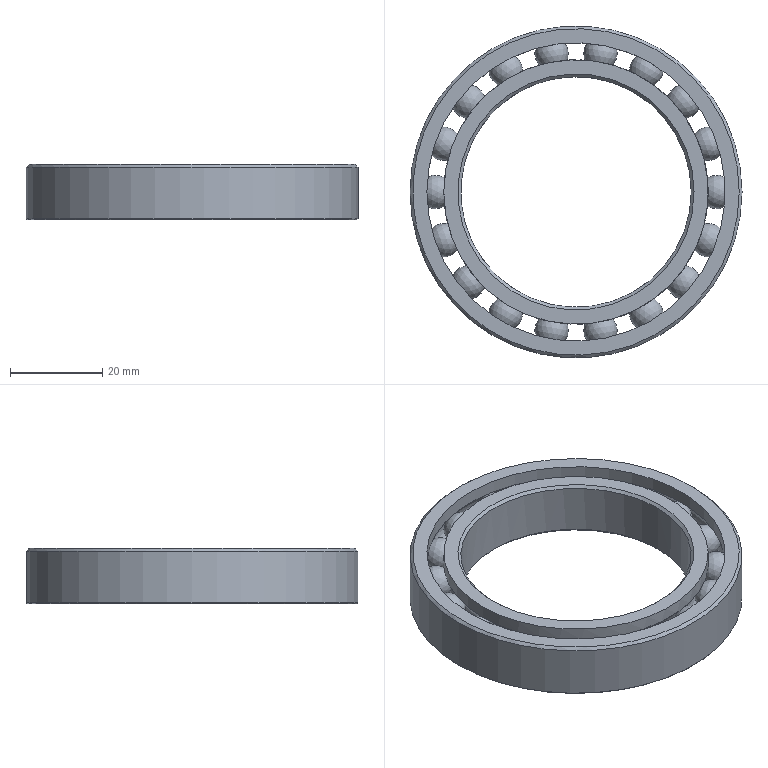Part | NX | 20 solids | 34 faces | box 72 x 72 x 12 mm | volume 17105 mm3 | sphere 18 | cylinder 5 | cone 5 | plane 4 | torus 2 | commonest cylinder face diameters 57.334 x2 50 x1 64.666 x1 72 x1
STEP:
#1=CARTESIAN_POINT('',(-5.296,-30.037,2.334));
#2=VERTEX_POINT('',#1);
#3=VERTEX_LOOP('',#2);
#4=FACE_BOUND('',#3,.T.);
#5=CARTESIAN_POINT('',(-5.296,-30.037,6.));
#6=DIRECTION('',(-0.1736,-0.9848,0.));
#7=DIRECTION('',(0.,0.,-1.));
#8=AXIS2_PLACEMENT_3D('',#5,#6,#7);
#9=SPHERICAL_SURFACE('',#8,3.666);
#10=ADVANCED_FACE('',(#4),#9,.T.);
#11=CLOSED_SHELL('',(#10));
#12=MANIFOLD_SOLID_BREP('',#11);
#13=CARTESIAN_POINT('',(5.296,30.037,2.334));
#14=VERTEX_POINT('',#13);
#15=VERTEX_LOOP('',#14);
#16=FACE_BOUND('',#15,.T.);
#17=CARTESIAN_POINT('',(5.296,30.037,6.));
#18=DIRECTION('',(0.1736,0.9848,0.));
#19=DIRECTION('',(0.,0.,-1.));
#20=AXIS2_PLACEMENT_3D('',#17,#18,#19);
#21=SPHERICAL_SURFACE('',#20,3.666);
#22=ADVANCED_FACE('',(#16),#21,.T.);
#23=CLOSED_SHELL('',(#22));
#24=MANIFOLD_SOLID_BREP('',#23);
#25=CARTESIAN_POINT('',(-23.364,19.605,2.334));
#26=VERTEX_POINT('',#25);
#27=VERTEX_LOOP('',#26);
#28=FACE_BOUND('',#27,.T.);
#29=CARTESIAN_POINT('',(-23.364,19.605,6.));
#30=DIRECTION('',(-0.766,0.6428,0.));
#31=DIRECTION('',(0.,0.,-1.));
#32=AXIS2_PLACEMENT_3D('',#29,#30,#31);
#33=SPHERICAL_SURFACE('',#32,3.666);
#34=ADVANCED_FACE('',(#28),#33,.T.);
#35=CLOSED_SHELL('',(#34));
#36=MANIFOLD_SOLID_BREP('',#35);
#37=CARTESIAN_POINT('',(28.661,10.432,2.334));
#38=VERTEX_POINT('',#37);
#39=VERTEX_LOOP('',#38);
#40=FACE_BOUND('',#39,.T.);
#41=CARTESIAN_POINT('',(28.661,10.432,6.));
#42=DIRECTION('',(0.9397,0.342,0.));
#43=DIRECTION('',(0.,0.,-1.));
#44=AXIS2_PLACEMENT_3D('',#41,#42,#43);
#45=SPHERICAL_SURFACE('',#44,3.666);
#46=ADVANCED_FACE('',(#40),#45,.T.);
#47=CLOSED_SHELL('',(#46));
#48=MANIFOLD_SOLID_BREP('',#47);
#49=CARTESIAN_POINT('',(-28.661,10.432,2.334));
#50=VERTEX_POINT('',#49);
#51=VERTEX_LOOP('',#50);
#52=FACE_BOUND('',#51,.T.);
#53=CARTESIAN_POINT('',(-28.661,10.432,6.));
#54=DIRECTION('',(-0.9397,0.342,0.));
#55=DIRECTION('',(0.,0.,-1.));
#56=AXIS2_PLACEMENT_3D('',#53,#54,#55);
#57=SPHERICAL_SURFACE('',#56,3.666);
#58=ADVANCED_FACE('',(#52),#57,.T.);
#59=CLOSED_SHELL('',(#58));
#60=MANIFOLD_SOLID_BREP('',#59);
#61=CARTESIAN_POINT('',(-23.364,-19.605,2.334));
#62=VERTEX_POINT('',#61);
#63=VERTEX_LOOP('',#62);
#64=FACE_BOUND('',#63,.T.);
#65=CARTESIAN_POINT('',(-23.364,-19.605,6.));
#66=DIRECTION('',(-0.766,-0.6428,0.));
#67=DIRECTION('',(0.,0.,-1.));
#68=AXIS2_PLACEMENT_3D('',#65,#66,#67);
#69=SPHERICAL_SURFACE('',#68,3.666);
#70=ADVANCED_FACE('',(#64),#69,.T.);
#71=CLOSED_SHELL('',(#70));
#72=MANIFOLD_SOLID_BREP('',#71);
#73=CARTESIAN_POINT('',(23.364,-19.605,2.334));
#74=VERTEX_POINT('',#73);
#75=VERTEX_LOOP('',#74);
#76=FACE_BOUND('',#75,.T.);
#77=CARTESIAN_POINT('',(23.364,-19.605,6.));
#78=DIRECTION('',(0.766,-0.6428,0.));
#79=DIRECTION('',(0.,0.,-1.));
#80=AXIS2_PLACEMENT_3D('',#77,#78,#79);
#81=SPHERICAL_SURFACE('',#80,3.666);
#82=ADVANCED_FACE('',(#76),#81,.T.);
#83=CLOSED_SHELL('',(#82));
#84=MANIFOLD_SOLID_BREP('',#83);
#85=CARTESIAN_POINT('',(15.25,-26.414,2.334));
#86=VERTEX_POINT('',#85);
#87=VERTEX_LOOP('',#86);
#88=FACE_BOUND('',#87,.T.);
#89=CARTESIAN_POINT('',(15.25,-26.414,6.));
#90=DIRECTION('',(0.5,-0.866,0.));
#91=DIRECTION('',(0.,0.,-1.));
#92=AXIS2_PLACEMENT_3D('',#89,#90,#91);
#93=SPHERICAL_SURFACE('',#92,3.666);
#94=ADVANCED_FACE('',(#88),#93,.T.);
#95=CLOSED_SHELL('',(#94));
#96=MANIFOLD_SOLID_BREP('',#95);
#97=CARTESIAN_POINT('',(-28.661,-10.432,2.334));
#98=VERTEX_POINT('',#97);
#99=VERTEX_LOOP('',#98);
#100=FACE_BOUND('',#99,.T.);
#101=CARTESIAN_POINT('',(-28.661,-10.432,6.));
#102=DIRECTION('',(-0.9397,-0.342,0.));
#103=DIRECTION('',(0.,0.,-1.));
#104=AXIS2_PLACEMENT_3D('',#101,#102,#103);
#105=SPHERICAL_SURFACE('',#104,3.666);
#106=ADVANCED_FACE('',(#100),#105,.T.);
#107=CLOSED_SHELL('',(#106));
#108=MANIFOLD_SOLID_BREP('',#107);
#109=CARTESIAN_POINT('',(-5.296,30.037,2.334));
#110=VERTEX_POINT('',#109);
#111=VERTEX_LOOP('',#110);
#112=FACE_BOUND('',#111,.T.);
#113=CARTESIAN_POINT('',(-5.296,30.037,6.));
#114=DIRECTION('',(-0.1736,0.9848,0.));
#115=DIRECTION('',(0.,0.,-1.));
#116=AXIS2_PLACEMENT_3D('',#113,#114,#115);
#117=SPHERICAL_SURFACE('',#116,3.666);
#118=ADVANCED_FACE('',(#112),#117,.T.);
#119=CLOSED_SHELL('',(#118));
#120=MANIFOLD_SOLID_BREP('',#119);
#121=CARTESIAN_POINT('',(15.25,26.414,2.334));
#122=VERTEX_POINT('',#121);
#123=VERTEX_LOOP('',#122);
#124=FACE_BOUND('',#123,.T.);
#125=CARTESIAN_POINT('',(15.25,26.414,6.));
#126=DIRECTION('',(0.5,0.866,0.));
#127=DIRECTION('',(0.,0.,-1.));
#128=AXIS2_PLACEMENT_3D('',#125,#126,#127);
#129=SPHERICAL_SURFACE('',#128,3.666);
#130=ADVANCED_FACE('',(#124),#129,.T.);
#131=CLOSED_SHELL('',(#130));
#132=MANIFOLD_SOLID_BREP('',#131);
#133=CARTESIAN_POINT('',(5.296,-30.037,2.334));
#134=VERTEX_POINT('',#133);
#135=VERTEX_LOOP('',#134);
#136=FACE_BOUND('',#135,.T.);
#137=CARTESIAN_POINT('',(5.296,-30.037,6.));
#138=DIRECTION('',(0.1736,-0.9848,0.));
#139=DIRECTION('',(0.,0.,-1.));
#140=AXIS2_PLACEMENT_3D('',#137,#138,#139);
#141=SPHERICAL_SURFACE('',#140,3.666);
#142=ADVANCED_FACE('',(#136),#141,.T.);
#143=CLOSED_SHELL('',(#142));
#144=MANIFOLD_SOLID_BREP('',#143);
#145=CARTESIAN_POINT('',(28.661,-10.432,2.334));
#146=VERTEX_POINT('',#145);
#147=VERTEX_LOOP('',#146);
#148=FACE_BOUND('',#147,.T.);
#149=CARTESIAN_POINT('',(28.661,-10.432,6.));
#150=DIRECTION('',(0.9397,-0.342,0.));
#151=DIRECTION('',(0.,0.,-1.));
#152=AXIS2_PLACEMENT_3D('',#149,#150,#151);
#153=SPHERICAL_SURFACE('',#152,3.666);
#154=ADVANCED_FACE('',(#148),#153,.T.);
#155=CLOSED_SHELL('',(#154));
#156=MANIFOLD_SOLID_BREP('',#155);
#157=CARTESIAN_POINT('',(-30.5,0.,2.334));
#158=VERTEX_POINT('',#157);
#159=VERTEX_LOOP('',#158);
#160=FACE_BOUND('',#159,.T.);
#161=CARTESIAN_POINT('',(-30.5,0.,6.));
#162=DIRECTION('',(-1.,0.,0.));
#163=DIRECTION('',(0.,0.,-1.));
#164=AXIS2_PLACEMENT_3D('',#161,#162,#163);
#165=SPHERICAL_SURFACE('',#164,3.666);
#166=ADVANCED_FACE('',(#160),#165,.T.);
#167=CLOSED_SHELL('',(#166));
#168=MANIFOLD_SOLID_BREP('',#167);
#169=CARTESIAN_POINT('',(23.364,19.605,2.334));
#170=VERTEX_POINT('',#169);
#171=VERTEX_LOOP('',#170);
#172=FACE_BOUND('',#171,.T.);
#173=CARTESIAN_POINT('',(23.364,19.605,6.));
#174=DIRECTION('',(0.766,0.6428,0.));
#175=DIRECTION('',(0.,0.,-1.));
#176=AXIS2_PLACEMENT_3D('',#173,#174,#175);
#177=SPHERICAL_SURFACE('',#176,3.666);
#178=ADVANCED_FACE('',(#172),#177,.T.);
#179=CLOSED_SHELL('',(#178));
#180=MANIFOLD_SOLID_BREP('',#179);
#181=CARTESIAN_POINT('',(-36.,0.,0.15));
#182=VERTEX_POINT('',#181);
#183=CARTESIAN_POINT('',(0.,0.,0.15));
#184=DIRECTION('',(0.,0.,1.));
#185=DIRECTION('',(-1.,0.,0.));
#186=AXIS2_PLACEMENT_3D('',#183,#184,#185);
#187=CIRCLE('',#186,36.);
#188=EDGE_CURVE('',#182,#182,#187,.T.);
#189=ORIENTED_EDGE('',*,*,#188,.T.);
#190=EDGE_LOOP('',(#189));
#191=FACE_BOUND('',#190,.T.);
#192=CARTESIAN_POINT('',(36.,0.,11.4));
#193=VERTEX_POINT('',#192);
#194=CARTESIAN_POINT('',(0.,0.,11.4));
#195=DIRECTION('',(0.,0.,-1.));
#196=DIRECTION('',(1.,0.,0.));
#197=AXIS2_PLACEMENT_3D('',#194,#195,#196);
#198=CIRCLE('',#197,36.);
#199=EDGE_CURVE('',#193,#193,#198,.T.);
#200=ORIENTED_EDGE('',*,*,#199,.T.);
#201=EDGE_LOOP('',(#200));
#202=FACE_BOUND('',#201,.T.);
#203=CARTESIAN_POINT('',(0.,0.,0.));
#204=DIRECTION('',(0.,0.,-1.));
#205=DIRECTION('',(1.,0.,0.));
#206=AXIS2_PLACEMENT_3D('',#203,#204,#205);
#207=CYLINDRICAL_SURFACE('',#206,36.);
#208=ADVANCED_FACE('',(#191,#202),#207,.T.);
#209=CARTESIAN_POINT('',(35.4,0.,12.));
#210=VERTEX_POINT('',#209);
#211=CARTESIAN_POINT('',(0.,0.,12.));
#212=DIRECTION('',(0.,0.,1.));
#213=DIRECTION('',(1.,0.,0.));
#214=AXIS2_PLACEMENT_3D('',#211,#212,#213);
#215=CIRCLE('',#214,35.4);
#216=EDGE_CURVE('',#210,#210,#215,.T.);
#217=ORIENTED_EDGE('',*,*,#216,.T.);
#218=EDGE_LOOP('',(#217));
#219=FACE_BOUND('',#218,.T.);
#220=CARTESIAN_POINT('',(-32.333,0.,12.));
#221=VERTEX_POINT('',#220);
#222=CARTESIAN_POINT('',(0.,0.,12.));
#223=DIRECTION('',(0.,0.,-1.));
#224=DIRECTION('',(-1.,0.,0.));
#225=AXIS2_PLACEMENT_3D('',#222,#223,#224);
#226=CIRCLE('',#225,32.333);
#227=EDGE_CURVE('',#221,#221,#226,.T.);
#228=ORIENTED_EDGE('',*,*,#227,.T.);
#229=EDGE_LOOP('',(#228));
#230=FACE_BOUND('',#229,.T.);
#231=CARTESIAN_POINT('',(36.,0.,12.));
#232=DIRECTION('',(0.,0.,1.));
#233=DIRECTION('',(-1.,0.,0.));
#234=AXIS2_PLACEMENT_3D('',#231,#232,#233);
#235=PLANE('',#234);
#236=ADVANCED_FACE('',(#219,#230),#235,.T.);
#237=CARTESIAN_POINT('',(-32.333,0.,9.175));
#238=VERTEX_POINT('',#237);
#239=CARTESIAN_POINT('',(0.,0.,9.175));
#240=DIRECTION('',(0.,0.,1.));
#241=DIRECTION('',(-1.,0.,0.));
#242=AXIS2_PLACEMENT_3D('',#239,#240,#241);
#243=CIRCLE('',#242,32.333);
#244=EDGE_CURVE('',#238,#238,#243,.T.);
#245=ORIENTED_EDGE('',*,*,#244,.F.);
#246=EDGE_LOOP('',(#245));
#247=FACE_BOUND('',#246,.T.);
#248=ORIENTED_EDGE('',*,*,#227,.F.);
#249=EDGE_LOOP('',(#248));
#250=FACE_BOUND('',#249,.T.);
#251=CARTESIAN_POINT('',(0.,0.,0.));
#252=DIRECTION('',(0.,0.,-1.));
#253=DIRECTION('',(1.,0.,0.));
#254=AXIS2_PLACEMENT_3D('',#251,#252,#253);
#255=CYLINDRICAL_SURFACE('',#254,32.333);
#256=ADVANCED_FACE('',(#247,#250),#255,.F.);
#257=CARTESIAN_POINT('',(-35.85,0.,0.));
#258=VERTEX_POINT('',#257);
#259=CARTESIAN_POINT('',(0.,0.,0.));
#260=DIRECTION('',(0.,0.,-1.));
#261=DIRECTION('',(-1.,0.,0.));
#262=AXIS2_PLACEMENT_3D('',#259,#260,#261);
#263=CIRCLE('',#262,35.85);
#264=EDGE_CURVE('',#258,#258,#263,.T.);
#265=ORIENTED_EDGE('',*,*,#264,.T.);
#266=EDGE_LOOP('',(#265));
#267=FACE_BOUND('',#266,.T.);
#268=CARTESIAN_POINT('',(-33.066,0.,0.));
#269=VERTEX_POINT('',#268);
#270=CARTESIAN_POINT('',(0.,0.,0.));
#271=DIRECTION('',(0.,0.,-1.));
#272=DIRECTION('',(-1.,0.,0.));
#273=AXIS2_PLACEMENT_3D('',#270,#271,#272);
#274=CIRCLE('',#273,33.066);
#275=EDGE_CURVE('',#269,#269,#274,.T.);
#276=ORIENTED_EDGE('',*,*,#275,.F.);
#277=EDGE_LOOP('',(#276));
#278=FACE_BOUND('',#277,.T.);
#279=CARTESIAN_POINT('',(32.333,0.,0.));
#280=DIRECTION('',(0.,0.,-1.));
#281=DIRECTION('',(1.,0.,0.));
#282=AXIS2_PLACEMENT_3D('',#279,#280,#281);
#283=PLANE('',#282);
#284=ADVANCED_FACE('',(#267,#278),#283,.T.);
#285=CARTESIAN_POINT('',(-32.333,0.,2.825));
#286=VERTEX_POINT('',#285);
#287=CARTESIAN_POINT('',(0.,0.,2.825));
#288=DIRECTION('',(0.,0.,-1.));
#289=DIRECTION('',(-1.,0.,0.));
#290=AXIS2_PLACEMENT_3D('',#287,#288,#289);
#291=CIRCLE('',#290,32.333);
#292=EDGE_CURVE('',#286,#286,#291,.T.);
#293=ORIENTED_EDGE('',*,*,#292,.T.);
#294=EDGE_LOOP('',(#293));
#295=FACE_BOUND('',#294,.T.);
#296=ORIENTED_EDGE('',*,*,#244,.T.);
#297=EDGE_LOOP('',(#296));
#298=FACE_BOUND('',#297,.T.);
#299=CARTESIAN_POINT('',(0.,0.,6.));
#300=DIRECTION('',(0.,0.,-1.));
#301=DIRECTION('',(1.,0.,0.));
#302=AXIS2_PLACEMENT_3D('',#299,#300,#301);
#303=TOROIDAL_SURFACE('',#302,30.5,3.666);
#304=ADVANCED_FACE('',(#295,#298),#303,.F.);
#305=ORIENTED_EDGE('',*,*,#292,.F.);
#306=EDGE_LOOP('',(#305));
#307=FACE_BOUND('',#306,.T.);
#308=ORIENTED_EDGE('',*,*,#275,.T.);
#309=EDGE_LOOP('',(#308));
#310=FACE_BOUND('',#309,.T.);
#311=CARTESIAN_POINT('',(0.,0.,0.));
#312=DIRECTION('',(0.,0.,-1.));
#313=DIRECTION('',(1.,0.,0.));
#314=AXIS2_PLACEMENT_3D('',#311,#312,#313);
#315=CONICAL_SURFACE('',#314,33.066,14.552);
#316=ADVANCED_FACE('',(#307,#310),#315,.F.);
#317=ORIENTED_EDGE('',*,*,#216,.F.);
#318=EDGE_LOOP('',(#317));
#319=FACE_BOUND('',#318,.T.);
#320=ORIENTED_EDGE('',*,*,#199,.F.);
#321=EDGE_LOOP('',(#320));
#322=FACE_BOUND('',#321,.T.);
#323=CARTESIAN_POINT('',(0.,0.,11.4));
#324=DIRECTION('',(0.,0.,-1.));
#325=DIRECTION('',(1.,0.,0.));
#326=AXIS2_PLACEMENT_3D('',#323,#324,#325);
#327=CONICAL_SURFACE('',#326,36.,45.);
#328=ADVANCED_FACE('',(#319,#322),#327,.T.);
#329=ORIENTED_EDGE('',*,*,#188,.F.);
#330=EDGE_LOOP('',(#329));
#331=FACE_BOUND('',#330,.T.);
#332=ORIENTED_EDGE('',*,*,#264,.F.);
#333=EDGE_LOOP('',(#332));
#334=FACE_BOUND('',#333,.T.);
#335=CARTESIAN_POINT('',(0.,0.,0.));
#336=DIRECTION('',(0.,0.,1.));
#337=DIRECTION('',(-1.,0.,0.));
#338=AXIS2_PLACEMENT_3D('',#335,#336,#337);
#339=CONICAL_SURFACE('',#338,35.85,45.);
#340=ADVANCED_FACE('',(#331,#334),#339,.T.);
#341=CLOSED_SHELL('',(#208,#236,#256,#284,#304,#316,#328,#340));
#342=MANIFOLD_SOLID_BREP('',#341);
#343=CARTESIAN_POINT('',(28.667,0.,2.825));
#344=VERTEX_POINT('',#343);
#345=CARTESIAN_POINT('',(0.,0.,2.825));
#346=DIRECTION('',(0.,0.,1.));
#347=DIRECTION('',(1.,0.,0.));
#348=AXIS2_PLACEMENT_3D('',#345,#346,#347);
#349=CIRCLE('',#348,28.667);
#350=EDGE_CURVE('',#344,#344,#349,.T.);
#351=ORIENTED_EDGE('',*,*,#350,.F.);
#352=EDGE_LOOP('',(#351));
#353=FACE_BOUND('',#352,.T.);
#354=CARTESIAN_POINT('',(-28.667,0.,0.));
#355=VERTEX_POINT('',#354);
#356=CARTESIAN_POINT('',(0.,0.,0.));
#357=DIRECTION('',(0.,0.,-1.));
#358=DIRECTION('',(-1.,0.,0.));
#359=AXIS2_PLACEMENT_3D('',#356,#357,#358);
#360=CIRCLE('',#359,28.667);
#361=EDGE_CURVE('',#355,#355,#360,.T.);
#362=ORIENTED_EDGE('',*,*,#361,.F.);
#363=EDGE_LOOP('',(#362));
#364=FACE_BOUND('',#363,.T.);
#365=CARTESIAN_POINT('',(0.,0.,0.));
#366=DIRECTION('',(0.,0.,-1.));
#367=DIRECTION('',(1.,0.,0.));
#368=AXIS2_PLACEMENT_3D('',#365,#366,#367);
#369=CYLINDRICAL_SURFACE('',#368,28.667);
#370=ADVANCED_FACE('',(#353,#364),#369,.T.);
#371=CARTESIAN_POINT('',(-25.,0.,0.6));
#372=VERTEX_POINT('',#371);
#373=CARTESIAN_POINT('',(0.,0.,0.6));
#374=DIRECTION('',(0.,0.,-1.));
#375=DIRECTION('',(-1.,0.,0.));
#376=AXIS2_PLACEMENT_3D('',#373,#374,#375);
#377=CIRCLE('',#376,25.);
#378=EDGE_CURVE('',#372,#372,#377,.T.);
#379=ORIENTED_EDGE('',*,*,#378,.T.);
#380=EDGE_LOOP('',(#379));
#381=FACE_BOUND('',#380,.T.);
#382=CARTESIAN_POINT('',(25.,0.,11.4));
#383=VERTEX_POINT('',#382);
#384=CARTESIAN_POINT('',(0.,0.,11.4));
#385=DIRECTION('',(0.,0.,1.));
#386=DIRECTION('',(1.,0.,0.));
#387=AXIS2_PLACEMENT_3D('',#384,#385,#386);
#388=CIRCLE('',#387,25.);
#389=EDGE_CURVE('',#383,#383,#388,.T.);
#390=ORIENTED_EDGE('',*,*,#389,.T.);
#391=EDGE_LOOP('',(#390));
#392=FACE_BOUND('',#391,.T.);
#393=CARTESIAN_POINT('',(0.,0.,0.));
#394=DIRECTION('',(0.,0.,-1.));
#395=DIRECTION('',(1.,0.,0.));
#396=AXIS2_PLACEMENT_3D('',#393,#394,#395);
#397=CYLINDRICAL_SURFACE('',#396,25.);
#398=ADVANCED_FACE('',(#381,#392),#397,.F.);
#399=CARTESIAN_POINT('',(-25.6,0.,0.));
#400=VERTEX_POINT('',#399);
#401=CARTESIAN_POINT('',(0.,0.,0.));
#402=DIRECTION('',(0.,0.,1.));
#403=DIRECTION('',(-1.,0.,0.));
#404=AXIS2_PLACEMENT_3D('',#401,#402,#403);
#405=CIRCLE('',#404,25.6);
#406=EDGE_CURVE('',#400,#400,#405,.T.);
#407=ORIENTED_EDGE('',*,*,#406,.T.);
#408=EDGE_LOOP('',(#407));
#409=FACE_BOUND('',#408,.T.);
#410=ORIENTED_EDGE('',*,*,#361,.T.);
#411=EDGE_LOOP('',(#410));
#412=FACE_BOUND('',#411,.T.);
#413=CARTESIAN_POINT('',(25.,0.,0.));
#414=DIRECTION('',(0.,0.,-1.));
#415=DIRECTION('',(1.,0.,0.));
#416=AXIS2_PLACEMENT_3D('',#413,#414,#415);
#417=PLANE('',#416);
#418=ADVANCED_FACE('',(#409,#412),#417,.T.);
#419=CARTESIAN_POINT('',(-28.667,0.,9.175));
#420=VERTEX_POINT('',#419);
#421=CARTESIAN_POINT('',(0.,0.,9.175));
#422=DIRECTION('',(0.,0.,-1.));
#423=DIRECTION('',(-1.,0.,0.));
#424=AXIS2_PLACEMENT_3D('',#421,#422,#423);
#425=CIRCLE('',#424,28.667);
#426=EDGE_CURVE('',#420,#420,#425,.T.);
#427=ORIENTED_EDGE('',*,*,#426,.F.);
#428=EDGE_LOOP('',(#427));
#429=FACE_BOUND('',#428,.T.);
#430=CARTESIAN_POINT('',(-28.667,0.,12.));
#431=VERTEX_POINT('',#430);
#432=CARTESIAN_POINT('',(0.,0.,12.));
#433=DIRECTION('',(0.,0.,-1.));
#434=DIRECTION('',(-1.,0.,0.));
#435=AXIS2_PLACEMENT_3D('',#432,#433,#434);
#436=CIRCLE('',#435,28.667);
#437=EDGE_CURVE('',#431,#431,#436,.T.);
#438=ORIENTED_EDGE('',*,*,#437,.T.);
#439=EDGE_LOOP('',(#438));
#440=FACE_BOUND('',#439,.T.);
#441=CARTESIAN_POINT('',(0.,0.,0.));
#442=DIRECTION('',(0.,0.,-1.));
#443=DIRECTION('',(1.,0.,0.));
#444=AXIS2_PLACEMENT_3D('',#441,#442,#443);
#445=CYLINDRICAL_SURFACE('',#444,28.667);
#446=ADVANCED_FACE('',(#429,#440),#445,.T.);
#447=CARTESIAN_POINT('',(25.6,0.,12.));
#448=VERTEX_POINT('',#447);
#449=CARTESIAN_POINT('',(0.,0.,12.));
#450=DIRECTION('',(0.,0.,-1.));
#451=DIRECTION('',(1.,0.,0.));
#452=AXIS2_PLACEMENT_3D('',#449,#450,#451);
#453=CIRCLE('',#452,25.6);
#454=EDGE_CURVE('',#448,#448,#453,.T.);
#455=ORIENTED_EDGE('',*,*,#454,.T.);
#456=EDGE_LOOP('',(#455));
#457=FACE_BOUND('',#456,.T.);
#458=ORIENTED_EDGE('',*,*,#437,.F.);
#459=EDGE_LOOP('',(#458));
#460=FACE_BOUND('',#459,.T.);
#461=CARTESIAN_POINT('',(28.667,0.,12.));
#462=DIRECTION('',(0.,0.,1.));
#463=DIRECTION('',(-1.,0.,0.));
#464=AXIS2_PLACEMENT_3D('',#461,#462,#463);
#465=PLANE('',#464);
#466=ADVANCED_FACE('',(#457,#460),#465,.T.);
#467=ORIENTED_EDGE('',*,*,#350,.T.);
#468=EDGE_LOOP('',(#467));
#469=FACE_BOUND('',#468,.T.);
#470=ORIENTED_EDGE('',*,*,#426,.T.);
#471=EDGE_LOOP('',(#470));
#472=FACE_BOUND('',#471,.T.);
#473=CARTESIAN_POINT('',(0.,0.,6.));
#474=DIRECTION('',(0.,0.,-1.));
#475=DIRECTION('',(1.,0.,0.));
#476=AXIS2_PLACEMENT_3D('',#473,#474,#475);
#477=TOROIDAL_SURFACE('',#476,30.5,3.666);
#478=ADVANCED_FACE('',(#469,#472),#477,.F.);
#479=ORIENTED_EDGE('',*,*,#406,.F.);
#480=EDGE_LOOP('',(#479));
#481=FACE_BOUND('',#480,.T.);
#482=ORIENTED_EDGE('',*,*,#378,.F.);
#483=EDGE_LOOP('',(#482));
#484=FACE_BOUND('',#483,.T.);
#485=CARTESIAN_POINT('',(0.,0.,0.6));
#486=DIRECTION('',(0.,0.,-1.));
#487=DIRECTION('',(1.,0.,0.));
#488=AXIS2_PLACEMENT_3D('',#485,#486,#487);
#489=CONICAL_SURFACE('',#488,25.,45.);
#490=ADVANCED_FACE('',(#481,#484),#489,.F.);
#491=ORIENTED_EDGE('',*,*,#389,.F.);
#492=EDGE_LOOP('',(#491));
#493=FACE_BOUND('',#492,.T.);
#494=ORIENTED_EDGE('',*,*,#454,.F.);
#495=EDGE_LOOP('',(#494));
#496=FACE_BOUND('',#495,.T.);
#497=CARTESIAN_POINT('',(0.,0.,12.));
#498=DIRECTION('',(0.,0.,1.));
#499=DIRECTION('',(-1.,0.,0.));
#500=AXIS2_PLACEMENT_3D('',#497,#498,#499);
#501=CONICAL_SURFACE('',#500,25.6,45.);
#502=ADVANCED_FACE('',(#493,#496),#501,.F.);
#503=CLOSED_SHELL('',(#370,#398,#418,#446,#466,#478,#490,#502));
#504=MANIFOLD_SOLID_BREP('',#503);
#505=CARTESIAN_POINT('',(-15.25,-26.414,2.334));
#506=VERTEX_POINT('',#505);
#507=VERTEX_LOOP('',#506);
#508=FACE_BOUND('',#507,.T.);
#509=CARTESIAN_POINT('',(-15.25,-26.414,6.));
#510=DIRECTION('',(-0.5,-0.866,0.));
#511=DIRECTION('',(0.,0.,-1.));
#512=AXIS2_PLACEMENT_3D('',#509,#510,#511);
#513=SPHERICAL_SURFACE('',#512,3.666);
#514=ADVANCED_FACE('',(#508),#513,.T.);
#515=CLOSED_SHELL('',(#514));
#516=MANIFOLD_SOLID_BREP('',#515);
#517=CARTESIAN_POINT('',(-15.25,26.414,2.334));
#518=VERTEX_POINT('',#517);
#519=VERTEX_LOOP('',#518);
#520=FACE_BOUND('',#519,.T.);
#521=CARTESIAN_POINT('',(-15.25,26.414,6.));
#522=DIRECTION('',(-0.5,0.866,0.));
#523=DIRECTION('',(0.,0.,-1.));
#524=AXIS2_PLACEMENT_3D('',#521,#522,#523);
#525=SPHERICAL_SURFACE('',#524,3.666);
#526=ADVANCED_FACE('',(#520),#525,.T.);
#527=CLOSED_SHELL('',(#526));
#528=MANIFOLD_SOLID_BREP('',#527);
#529=CARTESIAN_POINT('',(30.5,0.,2.334));
#530=VERTEX_POINT('',#529);
#531=VERTEX_LOOP('',#530);
#532=FACE_BOUND('',#531,.T.);
#533=CARTESIAN_POINT('',(30.5,0.,6.));
#534=DIRECTION('',(1.,0.,0.));
#535=DIRECTION('',(0.,0.,-1.));
#536=AXIS2_PLACEMENT_3D('',#533,#534,#535);
#537=SPHERICAL_SURFACE('',#536,3.666);
#538=ADVANCED_FACE('',(#532),#537,.T.);
#539=CLOSED_SHELL('',(#538));
#540=MANIFOLD_SOLID_BREP('',#539);
#541=(LENGTH_UNIT()NAMED_UNIT(*)SI_UNIT(.MILLI.,.METRE.));
#542=UNCERTAINTY_MEASURE_WITH_UNIT(LENGTH_MEASURE(0.00002),#541,'','');
#543=(NAMED_UNIT(*)PLANE_ANGLE_UNIT()SI_UNIT($,.RADIAN.));
#544=PLANE_ANGLE_MEASURE_WITH_UNIT(PLANE_ANGLE_MEASURE(0.01745),#543);
#545=DIMENSIONAL_EXPONENTS(0.,0.,0.,0.,0.,0.,0.);
#546=(CONVERSION_BASED_UNIT('DEGREE',#544)NAMED_UNIT(#545)PLANE_ANGLE_UNIT());
#547=(NAMED_UNIT(*)SI_UNIT($,.STERADIAN.)SOLID_ANGLE_UNIT());
#548=(GEOMETRIC_REPRESENTATION_CONTEXT(3)GLOBAL_UNCERTAINTY_ASSIGNED_CONTEXT((#542))GLOBAL_UNIT_ASSIGNED_CONTEXT((#541,#546,#547))REPRESENTATION_CONTEXT('',''));
#549=ADVANCED_BREP_SHAPE_REPRESENTATION('',(#12,#24,#36,#48,#60,#72,#84,#96,#108,#120,#132,#144,#156,#168,#180,#342,#504,#516,#528,#540),#548);